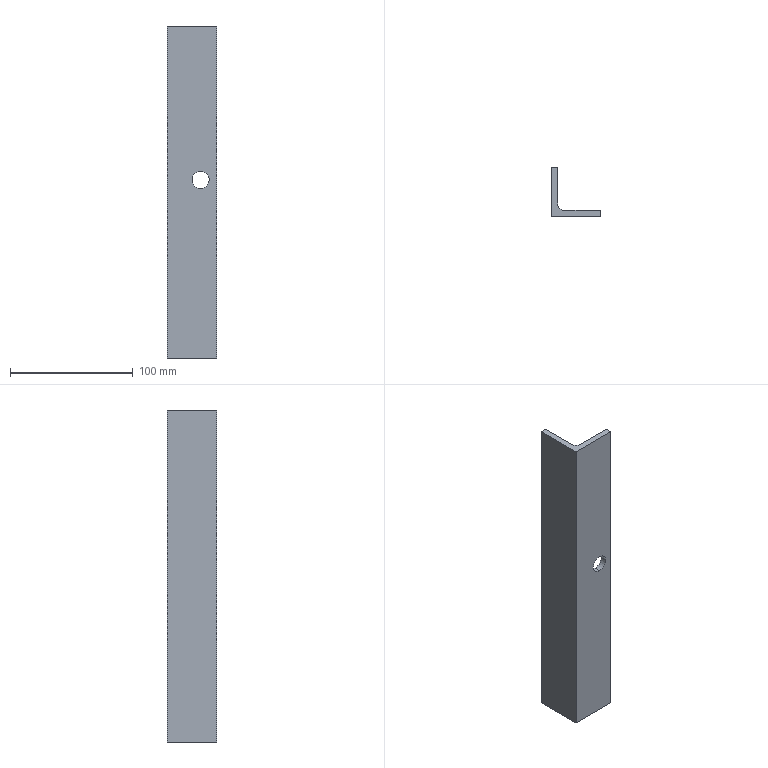Part | NX | features BREP 1 | 1 solid | 11 faces | box 40 x 40 x 270 mm | volume 101929 mm3 | plane 8 | cylinder 3 | commonest cylinder face diameters 14 x2 10 x1
STEP:
#1=CARTESIAN_POINT('',(27.,0.,3.));
#2=VERTEX_POINT('',#1);
#3=CARTESIAN_POINT('',(27.,0.,17.));
#4=VERTEX_POINT('',#3);
#5=CARTESIAN_POINT('',(27.,0.,10.));
#6=DIRECTION('',(0.,1.,0.));
#7=DIRECTION('',(0.,0.,1.));
#8=AXIS2_PLACEMENT_3D('',#5,#6,#7);
#9=CIRCLE('',#8,7.);
#10=EDGE_CURVE('',#2,#4,#9,.T.);
#11=ORIENTED_EDGE('',*,*,#10,.F.);
#12=CARTESIAN_POINT('',(27.,5.,3.));
#13=VERTEX_POINT('',#12);
#14=CARTESIAN_POINT('',(27.,0.,3.));
#15=DIRECTION('',(0.,1.,0.));
#16=VECTOR('',#15,1000.);
#17=LINE('',#14,#16);
#18=EDGE_CURVE('',#2,#13,#17,.T.);
#19=ORIENTED_EDGE('',*,*,#18,.T.);
#20=CARTESIAN_POINT('',(27.,5.,17.));
#21=VERTEX_POINT('',#20);
#22=CARTESIAN_POINT('',(27.,5.,10.));
#23=DIRECTION('',(0.,1.,0.));
#24=DIRECTION('',(0.,0.,1.));
#25=AXIS2_PLACEMENT_3D('',#22,#23,#24);
#26=CIRCLE('',#25,7.);
#27=EDGE_CURVE('',#13,#21,#26,.T.);
#28=ORIENTED_EDGE('',*,*,#27,.T.);
#29=CARTESIAN_POINT('',(27.,0.,17.));
#30=DIRECTION('',(0.,1.,0.));
#31=VECTOR('',#30,1000.);
#32=LINE('',#29,#31);
#33=EDGE_CURVE('',#4,#21,#32,.T.);
#34=ORIENTED_EDGE('',*,*,#33,.F.);
#35=EDGE_LOOP('',(#11,#19,#28,#34));
#36=FACE_BOUND('',#35,.T.);
#37=CARTESIAN_POINT('',(27.,0.,10.));
#38=DIRECTION('',(0.,1.,0.));
#39=DIRECTION('',(0.,0.,-1.));
#40=AXIS2_PLACEMENT_3D('',#37,#38,#39);
#41=CYLINDRICAL_SURFACE('',#40,7.);
#42=ADVANCED_FACE('',(#36),#41,.F.);
#43=CARTESIAN_POINT('',(40.,0.,-135.));
#44=VERTEX_POINT('',#43);
#45=CARTESIAN_POINT('',(40.,5.,-135.));
#46=VERTEX_POINT('',#45);
#47=CARTESIAN_POINT('',(40.,5.,-135.));
#48=DIRECTION('',(0.,1.,0.));
#49=VECTOR('',#48,1000.);
#50=LINE('',#47,#49);
#51=EDGE_CURVE('',#44,#46,#50,.T.);
#52=ORIENTED_EDGE('',*,*,#51,.T.);
#53=CARTESIAN_POINT('',(40.,5.,135.));
#54=VERTEX_POINT('',#53);
#55=CARTESIAN_POINT('',(40.,5.,135.));
#56=DIRECTION('',(0.,0.,-1.));
#57=VECTOR('',#56,1000.);
#58=LINE('',#55,#57);
#59=EDGE_CURVE('',#54,#46,#58,.T.);
#60=ORIENTED_EDGE('',*,*,#59,.F.);
#61=CARTESIAN_POINT('',(40.,0.,135.));
#62=VERTEX_POINT('',#61);
#63=CARTESIAN_POINT('',(40.,5.,135.));
#64=DIRECTION('',(0.,1.,0.));
#65=VECTOR('',#64,1000.);
#66=LINE('',#63,#65);
#67=EDGE_CURVE('',#62,#54,#66,.T.);
#68=ORIENTED_EDGE('',*,*,#67,.F.);
#69=CARTESIAN_POINT('',(40.,0.,135.));
#70=DIRECTION('',(0.,0.,-1.));
#71=VECTOR('',#70,1000.);
#72=LINE('',#69,#71);
#73=EDGE_CURVE('',#62,#44,#72,.T.);
#74=ORIENTED_EDGE('',*,*,#73,.T.);
#75=EDGE_LOOP('',(#52,#60,#68,#74));
#76=FACE_BOUND('',#75,.T.);
#77=CARTESIAN_POINT('',(40.,5.,135.));
#78=DIRECTION('',(-1.,0.,0.));
#79=DIRECTION('',(0.,0.,-1.));
#80=AXIS2_PLACEMENT_3D('',#77,#78,#79);
#81=PLANE('',#80);
#82=ADVANCED_FACE('',(#76),#81,.F.);
#83=CARTESIAN_POINT('',(27.,5.,10.));
#84=DIRECTION('',(0.,1.,0.));
#85=DIRECTION('',(0.,0.,1.));
#86=AXIS2_PLACEMENT_3D('',#83,#84,#85);
#87=CIRCLE('',#86,7.);
#88=EDGE_CURVE('',#21,#13,#87,.T.);
#89=ORIENTED_EDGE('',*,*,#88,.F.);
#90=ORIENTED_EDGE('',*,*,#27,.F.);
#91=EDGE_LOOP('',(#89,#90));
#92=FACE_BOUND('',#91,.T.);
#93=CARTESIAN_POINT('',(10.,5.,-135.));
#94=VERTEX_POINT('',#93);
#95=CARTESIAN_POINT('',(10.,5.,-135.));
#96=DIRECTION('',(-1.,0.,0.));
#97=VECTOR('',#96,1000.);
#98=LINE('',#95,#97);
#99=EDGE_CURVE('',#46,#94,#98,.T.);
#100=ORIENTED_EDGE('',*,*,#99,.T.);
#101=CARTESIAN_POINT('',(10.,5.,135.));
#102=VERTEX_POINT('',#101);
#103=CARTESIAN_POINT('',(10.,5.,135.));
#104=DIRECTION('',(0.,0.,-1.));
#105=VECTOR('',#104,1000.);
#106=LINE('',#103,#105);
#107=EDGE_CURVE('',#102,#94,#106,.T.);
#108=ORIENTED_EDGE('',*,*,#107,.F.);
#109=CARTESIAN_POINT('',(10.,5.,135.));
#110=DIRECTION('',(-1.,0.,0.));
#111=VECTOR('',#110,1000.);
#112=LINE('',#109,#111);
#113=EDGE_CURVE('',#54,#102,#112,.T.);
#114=ORIENTED_EDGE('',*,*,#113,.F.);
#115=ORIENTED_EDGE('',*,*,#59,.T.);
#116=EDGE_LOOP('',(#100,#108,#114,#115));
#117=FACE_BOUND('',#116,.T.);
#118=CARTESIAN_POINT('',(10.,5.,135.));
#119=DIRECTION('',(0.,-1.,0.));
#120=DIRECTION('',(0.,0.,1.));
#121=AXIS2_PLACEMENT_3D('',#118,#119,#120);
#122=PLANE('',#121);
#123=ADVANCED_FACE('',(#92,#117),#122,.F.);
#124=CARTESIAN_POINT('',(5.,10.,-135.));
#125=VERTEX_POINT('',#124);
#126=CARTESIAN_POINT('',(10.,10.,-135.));
#127=DIRECTION('',(0.,0.,-1.));
#128=DIRECTION('',(1.,0.,0.));
#129=AXIS2_PLACEMENT_3D('',#126,#127,#128);
#130=CIRCLE('',#129,5.);
#131=EDGE_CURVE('',#94,#125,#130,.T.);
#132=ORIENTED_EDGE('',*,*,#131,.T.);
#133=CARTESIAN_POINT('',(5.,10.,135.));
#134=VERTEX_POINT('',#133);
#135=CARTESIAN_POINT('',(5.,10.,135.));
#136=DIRECTION('',(0.,0.,-1.));
#137=VECTOR('',#136,1000.);
#138=LINE('',#135,#137);
#139=EDGE_CURVE('',#134,#125,#138,.T.);
#140=ORIENTED_EDGE('',*,*,#139,.F.);
#141=CARTESIAN_POINT('',(10.,10.,135.));
#142=DIRECTION('',(0.,0.,-1.));
#143=DIRECTION('',(1.,0.,0.));
#144=AXIS2_PLACEMENT_3D('',#141,#142,#143);
#145=CIRCLE('',#144,5.);
#146=EDGE_CURVE('',#102,#134,#145,.T.);
#147=ORIENTED_EDGE('',*,*,#146,.F.);
#148=ORIENTED_EDGE('',*,*,#107,.T.);
#149=EDGE_LOOP('',(#132,#140,#147,#148));
#150=FACE_BOUND('',#149,.T.);
#151=CARTESIAN_POINT('',(10.,10.,135.));
#152=DIRECTION('',(0.,0.,-1.));
#153=DIRECTION('',(1.,0.,0.));
#154=AXIS2_PLACEMENT_3D('',#151,#152,#153);
#155=CYLINDRICAL_SURFACE('',#154,5.);
#156=ADVANCED_FACE('',(#150),#155,.F.);
#157=CARTESIAN_POINT('',(5.,40.,-135.));
#158=VERTEX_POINT('',#157);
#159=CARTESIAN_POINT('',(5.,40.,-135.));
#160=DIRECTION('',(0.,1.,0.));
#161=VECTOR('',#160,1000.);
#162=LINE('',#159,#161);
#163=EDGE_CURVE('',#125,#158,#162,.T.);
#164=ORIENTED_EDGE('',*,*,#163,.T.);
#165=CARTESIAN_POINT('',(5.,40.,135.));
#166=VERTEX_POINT('',#165);
#167=CARTESIAN_POINT('',(5.,40.,135.));
#168=DIRECTION('',(0.,0.,-1.));
#169=VECTOR('',#168,1000.);
#170=LINE('',#167,#169);
#171=EDGE_CURVE('',#166,#158,#170,.T.);
#172=ORIENTED_EDGE('',*,*,#171,.F.);
#173=CARTESIAN_POINT('',(5.,40.,135.));
#174=DIRECTION('',(0.,1.,0.));
#175=VECTOR('',#174,1000.);
#176=LINE('',#173,#175);
#177=EDGE_CURVE('',#134,#166,#176,.T.);
#178=ORIENTED_EDGE('',*,*,#177,.F.);
#179=ORIENTED_EDGE('',*,*,#139,.T.);
#180=EDGE_LOOP('',(#164,#172,#178,#179));
#181=FACE_BOUND('',#180,.T.);
#182=CARTESIAN_POINT('',(5.,40.,135.));
#183=DIRECTION('',(-1.,0.,0.));
#184=DIRECTION('',(0.,0.,-1.));
#185=AXIS2_PLACEMENT_3D('',#182,#183,#184);
#186=PLANE('',#185);
#187=ADVANCED_FACE('',(#181),#186,.F.);
#188=CARTESIAN_POINT('',(0.,40.,-135.));
#189=VERTEX_POINT('',#188);
#190=CARTESIAN_POINT('',(0.,40.,-135.));
#191=DIRECTION('',(-1.,0.,0.));
#192=VECTOR('',#191,1000.);
#193=LINE('',#190,#192);
#194=EDGE_CURVE('',#158,#189,#193,.T.);
#195=ORIENTED_EDGE('',*,*,#194,.T.);
#196=CARTESIAN_POINT('',(0.,40.,135.));
#197=VERTEX_POINT('',#196);
#198=CARTESIAN_POINT('',(0.,40.,135.));
#199=DIRECTION('',(0.,0.,-1.));
#200=VECTOR('',#199,1000.);
#201=LINE('',#198,#200);
#202=EDGE_CURVE('',#197,#189,#201,.T.);
#203=ORIENTED_EDGE('',*,*,#202,.F.);
#204=CARTESIAN_POINT('',(0.,40.,135.));
#205=DIRECTION('',(-1.,0.,0.));
#206=VECTOR('',#205,1000.);
#207=LINE('',#204,#206);
#208=EDGE_CURVE('',#166,#197,#207,.T.);
#209=ORIENTED_EDGE('',*,*,#208,.F.);
#210=ORIENTED_EDGE('',*,*,#171,.T.);
#211=EDGE_LOOP('',(#195,#203,#209,#210));
#212=FACE_BOUND('',#211,.T.);
#213=CARTESIAN_POINT('',(0.,40.,135.));
#214=DIRECTION('',(0.,-1.,0.));
#215=DIRECTION('',(0.,0.,1.));
#216=AXIS2_PLACEMENT_3D('',#213,#214,#215);
#217=PLANE('',#216);
#218=ADVANCED_FACE('',(#212),#217,.F.);
#219=CARTESIAN_POINT('',(0.,0.,-135.));
#220=VERTEX_POINT('',#219);
#221=CARTESIAN_POINT('',(0.,0.,-135.));
#222=DIRECTION('',(0.,-1.,0.));
#223=VECTOR('',#222,1000.);
#224=LINE('',#221,#223);
#225=EDGE_CURVE('',#189,#220,#224,.T.);
#226=ORIENTED_EDGE('',*,*,#225,.T.);
#227=CARTESIAN_POINT('',(0.,0.,135.));
#228=VERTEX_POINT('',#227);
#229=CARTESIAN_POINT('',(0.,0.,135.));
#230=DIRECTION('',(0.,0.,-1.));
#231=VECTOR('',#230,1000.);
#232=LINE('',#229,#231);
#233=EDGE_CURVE('',#228,#220,#232,.T.);
#234=ORIENTED_EDGE('',*,*,#233,.F.);
#235=CARTESIAN_POINT('',(0.,0.,135.));
#236=DIRECTION('',(0.,-1.,0.));
#237=VECTOR('',#236,1000.);
#238=LINE('',#235,#237);
#239=EDGE_CURVE('',#197,#228,#238,.T.);
#240=ORIENTED_EDGE('',*,*,#239,.F.);
#241=ORIENTED_EDGE('',*,*,#202,.T.);
#242=EDGE_LOOP('',(#226,#234,#240,#241));
#243=FACE_BOUND('',#242,.T.);
#244=CARTESIAN_POINT('',(0.,0.,135.));
#245=DIRECTION('',(1.,0.,0.));
#246=DIRECTION('',(0.,0.,1.));
#247=AXIS2_PLACEMENT_3D('',#244,#245,#246);
#248=PLANE('',#247);
#249=ADVANCED_FACE('',(#243),#248,.F.);
#250=CARTESIAN_POINT('',(27.,0.,10.));
#251=DIRECTION('',(0.,1.,0.));
#252=DIRECTION('',(0.,0.,1.));
#253=AXIS2_PLACEMENT_3D('',#250,#251,#252);
#254=CIRCLE('',#253,7.);
#255=EDGE_CURVE('',#4,#2,#254,.T.);
#256=ORIENTED_EDGE('',*,*,#255,.T.);
#257=ORIENTED_EDGE('',*,*,#10,.T.);
#258=EDGE_LOOP('',(#256,#257));
#259=FACE_BOUND('',#258,.T.);
#260=CARTESIAN_POINT('',(40.,0.,-135.));
#261=DIRECTION('',(1.,0.,0.));
#262=VECTOR('',#261,1000.);
#263=LINE('',#260,#262);
#264=EDGE_CURVE('',#220,#44,#263,.T.);
#265=ORIENTED_EDGE('',*,*,#264,.T.);
#266=ORIENTED_EDGE('',*,*,#73,.F.);
#267=CARTESIAN_POINT('',(40.,0.,135.));
#268=DIRECTION('',(1.,0.,0.));
#269=VECTOR('',#268,1000.);
#270=LINE('',#267,#269);
#271=EDGE_CURVE('',#228,#62,#270,.T.);
#272=ORIENTED_EDGE('',*,*,#271,.F.);
#273=ORIENTED_EDGE('',*,*,#233,.T.);
#274=EDGE_LOOP('',(#265,#266,#272,#273));
#275=FACE_BOUND('',#274,.T.);
#276=CARTESIAN_POINT('',(40.,0.,135.));
#277=DIRECTION('',(0.,1.,0.));
#278=DIRECTION('',(0.,0.,-1.));
#279=AXIS2_PLACEMENT_3D('',#276,#277,#278);
#280=PLANE('',#279);
#281=ADVANCED_FACE('',(#259,#275),#280,.F.);
#282=ORIENTED_EDGE('',*,*,#67,.T.);
#283=ORIENTED_EDGE('',*,*,#113,.T.);
#284=ORIENTED_EDGE('',*,*,#146,.T.);
#285=ORIENTED_EDGE('',*,*,#177,.T.);
#286=ORIENTED_EDGE('',*,*,#208,.T.);
#287=ORIENTED_EDGE('',*,*,#239,.T.);
#288=ORIENTED_EDGE('',*,*,#271,.T.);
#289=EDGE_LOOP('',(#282,#283,#284,#285,#286,#287,#288));
#290=FACE_BOUND('',#289,.T.);
#291=CARTESIAN_POINT('',(10.,10.,135.));
#292=DIRECTION('',(0.,0.,1.));
#293=DIRECTION('',(-1.,0.,0.));
#294=AXIS2_PLACEMENT_3D('',#291,#292,#293);
#295=PLANE('',#294);
#296=ADVANCED_FACE('',(#290),#295,.T.);
#297=ORIENTED_EDGE('',*,*,#51,.F.);
#298=ORIENTED_EDGE('',*,*,#264,.F.);
#299=ORIENTED_EDGE('',*,*,#225,.F.);
#300=ORIENTED_EDGE('',*,*,#194,.F.);
#301=ORIENTED_EDGE('',*,*,#163,.F.);
#302=ORIENTED_EDGE('',*,*,#131,.F.);
#303=ORIENTED_EDGE('',*,*,#99,.F.);
#304=EDGE_LOOP('',(#297,#298,#299,#300,#301,#302,#303));
#305=FACE_BOUND('',#304,.T.);
#306=CARTESIAN_POINT('',(10.,10.,-135.));
#307=DIRECTION('',(0.,0.,1.));
#308=DIRECTION('',(-1.,0.,0.));
#309=AXIS2_PLACEMENT_3D('',#306,#307,#308);
#310=PLANE('',#309);
#311=ADVANCED_FACE('',(#305),#310,.F.);
#312=ORIENTED_EDGE('',*,*,#18,.F.);
#313=ORIENTED_EDGE('',*,*,#255,.F.);
#314=ORIENTED_EDGE('',*,*,#33,.T.);
#315=ORIENTED_EDGE('',*,*,#88,.T.);
#316=EDGE_LOOP('',(#312,#313,#314,#315));
#317=FACE_BOUND('',#316,.T.);
#318=CARTESIAN_POINT('',(27.,0.,10.));
#319=DIRECTION('',(0.,1.,0.));
#320=DIRECTION('',(0.,0.,-1.));
#321=AXIS2_PLACEMENT_3D('',#318,#319,#320);
#322=CYLINDRICAL_SURFACE('',#321,7.);
#323=ADVANCED_FACE('',(#317),#322,.F.);
#324=CLOSED_SHELL('',(#42,#82,#123,#156,#187,#218,#249,#281,#296,#311,#323));
#325=MANIFOLD_SOLID_BREP('',#324);
#326=(LENGTH_UNIT()NAMED_UNIT(*)SI_UNIT(.MILLI.,.METRE.));
#327=UNCERTAINTY_MEASURE_WITH_UNIT(LENGTH_MEASURE(0.00001),#326,'','');
#328=(NAMED_UNIT(*)PLANE_ANGLE_UNIT()SI_UNIT($,.RADIAN.));
#329=(NAMED_UNIT(*)SI_UNIT($,.STERADIAN.)SOLID_ANGLE_UNIT());
#330=(GEOMETRIC_REPRESENTATION_CONTEXT(3)GLOBAL_UNCERTAINTY_ASSIGNED_CONTEXT((#327))GLOBAL_UNIT_ASSIGNED_CONTEXT((#326,#328,#329))REPRESENTATION_CONTEXT('',''));
#331=ADVANCED_BREP_SHAPE_REPRESENTATION('',(#325),#330);